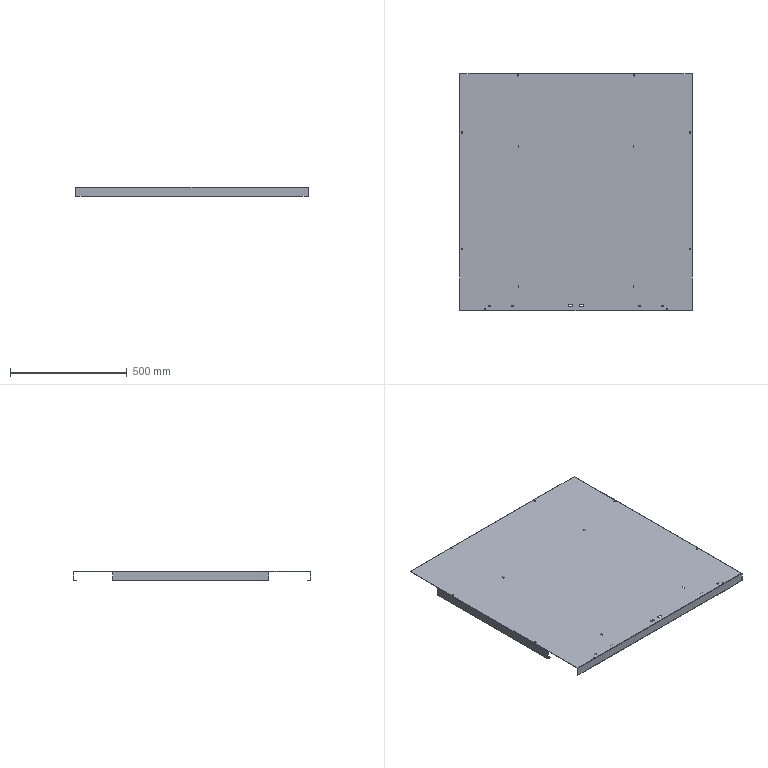Part | STEP file | FHD-021-001-A rack welded part A | 1 solid | 102 faces | box 1000 x 1020 x 40 mm | volume 1755209 mm3 | plane 74 | cylinder 28 | commonest cylinder face diameters 0.4 x8 3.4 x8 5.2 x4 6 x4 9 x4